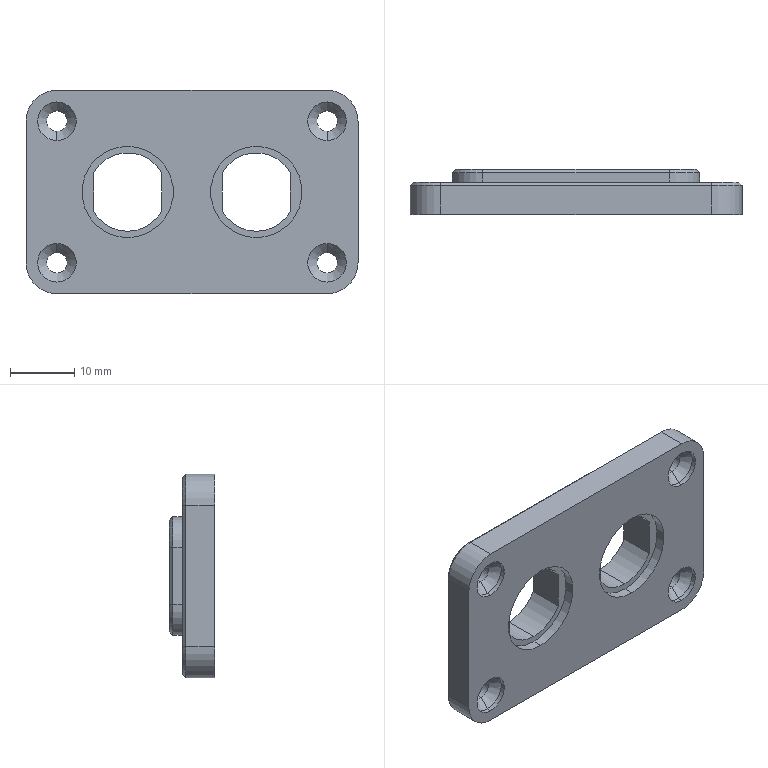Part | SolidWorks | features ICE 3, Chamfer 1, Extrusion 1, Fillet 1, HoleWzd 1 | 1 solid | 75 faces | box 51.6 x 7 x 31.6 mm | volume 7439 mm3 | cylinder 34 | plane 25 | cone 16 | commonest cylinder face diameters 3.2 x8 6 x8 12.2 x6 9.4 x4 9.6 x4 14.2 x4